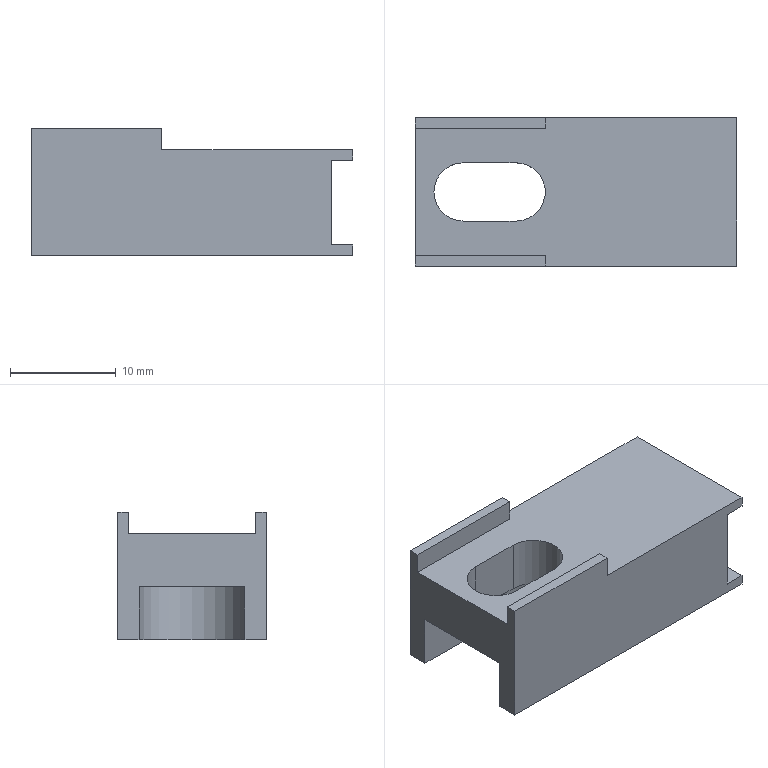Part | NX | features BREP 1 | 1 solid | 29 faces | box 30.3 x 14 x 12 mm | volume 3050 mm3 | plane 21 | cylinder 6 | cone 2 | commonest cylinder face diameters 5.5 x3 3.3 x2 10 x1
STEP:
#1=CARTESIAN_POINT('',(-758.104,11.58,6.65));
#2=VERTEX_POINT('',#1);
#3=CARTESIAN_POINT('',(-758.104,11.58,3.35));
#4=VERTEX_POINT('',#3);
#5=CARTESIAN_POINT('',(-758.104,11.58,5.));
#6=DIRECTION('',(1.,0.,0.));
#7=DIRECTION('',(0.,0.,-1.));
#8=AXIS2_PLACEMENT_3D('',#5,#6,#7);
#9=CIRCLE('',#8,1.65);
#10=EDGE_CURVE('',#2,#4,#9,.T.);
#11=ORIENTED_EDGE('',*,*,#10,.F.);
#12=CARTESIAN_POINT('',(-748.004,11.58,6.65));
#13=VERTEX_POINT('',#12);
#14=CARTESIAN_POINT('',(-748.004,11.58,6.65));
#15=DIRECTION('',(1.,0.,0.));
#16=VECTOR('',#15,1000.);
#17=LINE('',#14,#16);
#18=EDGE_CURVE('',#2,#13,#17,.T.);
#19=ORIENTED_EDGE('',*,*,#18,.T.);
#20=CARTESIAN_POINT('',(-748.004,11.58,3.35));
#21=VERTEX_POINT('',#20);
#22=CARTESIAN_POINT('',(-748.004,11.58,5.));
#23=DIRECTION('',(1.,0.,0.));
#24=DIRECTION('',(0.,0.,-1.));
#25=AXIS2_PLACEMENT_3D('',#22,#23,#24);
#26=CIRCLE('',#25,1.65);
#27=EDGE_CURVE('',#13,#21,#26,.T.);
#28=ORIENTED_EDGE('',*,*,#27,.T.);
#29=CARTESIAN_POINT('',(-748.004,11.58,3.35));
#30=DIRECTION('',(1.,0.,0.));
#31=VECTOR('',#30,1000.);
#32=LINE('',#29,#31);
#33=EDGE_CURVE('',#4,#21,#32,.T.);
#34=ORIENTED_EDGE('',*,*,#33,.F.);
#35=EDGE_LOOP('',(#11,#19,#28,#34));
#36=FACE_BOUND('',#35,.T.);
#37=CARTESIAN_POINT('',(-748.004,11.58,5.));
#38=DIRECTION('',(1.,0.,0.));
#39=DIRECTION('',(0.,0.,-1.));
#40=AXIS2_PLACEMENT_3D('',#37,#38,#39);
#41=CYLINDRICAL_SURFACE('',#40,1.65);
#42=ADVANCED_FACE('',(#36),#41,.F.);
#43=CARTESIAN_POINT('',(-759.096,11.58,5.));
#44=VERTEX_POINT('',#43);
#45=CARTESIAN_POINT('',(-758.104,11.58,3.35));
#46=DIRECTION('',(0.515,0.,-0.8572));
#47=VECTOR('',#46,1000.);
#48=LINE('',#45,#47);
#49=EDGE_CURVE('',#44,#4,#48,.T.);
#50=ORIENTED_EDGE('',*,*,#49,.F.);
#51=CARTESIAN_POINT('',(-758.104,11.58,6.65));
#52=DIRECTION('',(0.515,0.,0.8572));
#53=VECTOR('',#52,1000.);
#54=LINE('',#51,#53);
#55=EDGE_CURVE('',#44,#2,#54,.T.);
#56=ORIENTED_EDGE('',*,*,#55,.T.);
#57=ORIENTED_EDGE('',*,*,#10,.T.);
#58=EDGE_LOOP('',(#50,#56,#57));
#59=FACE_BOUND('',#58,.T.);
#60=CARTESIAN_POINT('',(-758.104,11.58,5.));
#61=DIRECTION('',(1.,0.,0.));
#62=DIRECTION('',(0.,0.,-1.));
#63=AXIS2_PLACEMENT_3D('',#60,#61,#62);
#64=CONICAL_SURFACE('',#63,1.65,1.03);
#65=ADVANCED_FACE('',(#59),#64,.F.);
#66=CARTESIAN_POINT('',(-774.554,11.58,10.));
#67=VERTEX_POINT('',#66);
#68=CARTESIAN_POINT('',(-771.804,14.33,10.));
#69=VERTEX_POINT('',#68);
#70=CARTESIAN_POINT('',(-771.804,11.58,10.));
#71=DIRECTION('',(0.,0.,-1.));
#72=DIRECTION('',(-1.,0.,0.));
#73=AXIS2_PLACEMENT_3D('',#70,#71,#72);
#74=CIRCLE('',#73,2.75);
#75=EDGE_CURVE('',#67,#69,#74,.T.);
#76=ORIENTED_EDGE('',*,*,#75,.F.);
#77=CARTESIAN_POINT('',(-774.554,11.58,5.));
#78=VERTEX_POINT('',#77);
#79=CARTESIAN_POINT('',(-774.554,11.58,12.));
#80=DIRECTION('',(0.,0.,-1.));
#81=VECTOR('',#80,1000.);
#82=LINE('',#79,#81);
#83=EDGE_CURVE('',#67,#78,#82,.T.);
#84=ORIENTED_EDGE('',*,*,#83,.T.);
#85=CARTESIAN_POINT('',(-771.804,14.33,5.));
#86=VERTEX_POINT('',#85);
#87=CARTESIAN_POINT('',(-771.804,11.58,5.));
#88=DIRECTION('',(0.,0.,1.));
#89=DIRECTION('',(-1.,0.,0.));
#90=AXIS2_PLACEMENT_3D('',#87,#88,#89);
#91=CIRCLE('',#90,2.75);
#92=EDGE_CURVE('',#86,#78,#91,.T.);
#93=ORIENTED_EDGE('',*,*,#92,.F.);
#94=CARTESIAN_POINT('',(-771.804,14.33,12.));
#95=DIRECTION('',(0.,0.,-1.));
#96=VECTOR('',#95,1000.);
#97=LINE('',#94,#96);
#98=EDGE_CURVE('',#69,#86,#97,.T.);
#99=ORIENTED_EDGE('',*,*,#98,.F.);
#100=EDGE_LOOP('',(#76,#84,#93,#99));
#101=FACE_BOUND('',#100,.T.);
#102=CARTESIAN_POINT('',(-771.804,11.58,12.));
#103=DIRECTION('',(0.,0.,-1.));
#104=DIRECTION('',(-1.,0.,0.));
#105=AXIS2_PLACEMENT_3D('',#102,#103,#104);
#106=CYLINDRICAL_SURFACE('',#105,2.75);
#107=ADVANCED_FACE('',(#101),#106,.F.);
#108=CARTESIAN_POINT('',(-776.304,16.58,0.));
#109=VERTEX_POINT('',#108);
#110=CARTESIAN_POINT('',(-776.304,16.58,5.));
#111=VERTEX_POINT('',#110);
#112=CARTESIAN_POINT('',(-776.304,16.58,0.));
#113=DIRECTION('',(0.,0.,1.));
#114=VECTOR('',#113,1000.);
#115=LINE('',#112,#114);
#116=EDGE_CURVE('',#109,#111,#115,.T.);
#117=ORIENTED_EDGE('',*,*,#116,.T.);
#118=CARTESIAN_POINT('',(-776.304,6.58,5.));
#119=VERTEX_POINT('',#118);
#120=CARTESIAN_POINT('',(-776.304,18.58,5.));
#121=DIRECTION('',(0.,1.,0.));
#122=VECTOR('',#121,1000.);
#123=LINE('',#120,#122);
#124=EDGE_CURVE('',#119,#111,#123,.T.);
#125=ORIENTED_EDGE('',*,*,#124,.F.);
#126=CARTESIAN_POINT('',(-776.304,6.58,0.));
#127=VERTEX_POINT('',#126);
#128=CARTESIAN_POINT('',(-776.304,6.58,0.));
#129=DIRECTION('',(0.,0.,1.));
#130=VECTOR('',#129,1000.);
#131=LINE('',#128,#130);
#132=EDGE_CURVE('',#127,#119,#131,.T.);
#133=ORIENTED_EDGE('',*,*,#132,.F.);
#134=CARTESIAN_POINT('',(-776.304,4.58,0.));
#135=VERTEX_POINT('',#134);
#136=CARTESIAN_POINT('',(-776.304,18.58,0.));
#137=DIRECTION('',(0.,-1.,0.));
#138=VECTOR('',#137,1000.);
#139=LINE('',#136,#138);
#140=EDGE_CURVE('',#127,#135,#139,.T.);
#141=ORIENTED_EDGE('',*,*,#140,.T.);
#142=CARTESIAN_POINT('',(-776.304,4.58,12.));
#143=VERTEX_POINT('',#142);
#144=CARTESIAN_POINT('',(-776.304,4.58,12.));
#145=DIRECTION('',(0.,0.,-1.));
#146=VECTOR('',#145,1000.);
#147=LINE('',#144,#146);
#148=EDGE_CURVE('',#143,#135,#147,.T.);
#149=ORIENTED_EDGE('',*,*,#148,.F.);
#150=CARTESIAN_POINT('',(-776.304,5.58,12.));
#151=VERTEX_POINT('',#150);
#152=CARTESIAN_POINT('',(-776.304,18.58,12.));
#153=DIRECTION('',(0.,-1.,0.));
#154=VECTOR('',#153,1000.);
#155=LINE('',#152,#154);
#156=EDGE_CURVE('',#151,#143,#155,.T.);
#157=ORIENTED_EDGE('',*,*,#156,.F.);
#158=CARTESIAN_POINT('',(-776.304,5.58,10.));
#159=VERTEX_POINT('',#158);
#160=CARTESIAN_POINT('',(-776.304,5.58,10.));
#161=DIRECTION('',(0.,0.,1.));
#162=VECTOR('',#161,1000.);
#163=LINE('',#160,#162);
#164=EDGE_CURVE('',#159,#151,#163,.T.);
#165=ORIENTED_EDGE('',*,*,#164,.F.);
#166=CARTESIAN_POINT('',(-776.304,17.58,10.));
#167=VERTEX_POINT('',#166);
#168=CARTESIAN_POINT('',(-776.304,5.58,10.));
#169=DIRECTION('',(0.,-1.,0.));
#170=VECTOR('',#169,1000.);
#171=LINE('',#168,#170);
#172=EDGE_CURVE('',#167,#159,#171,.T.);
#173=ORIENTED_EDGE('',*,*,#172,.F.);
#174=CARTESIAN_POINT('',(-776.304,17.58,12.));
#175=VERTEX_POINT('',#174);
#176=CARTESIAN_POINT('',(-776.304,17.58,10.));
#177=DIRECTION('',(0.,0.,1.));
#178=VECTOR('',#177,1000.);
#179=LINE('',#176,#178);
#180=EDGE_CURVE('',#167,#175,#179,.T.);
#181=ORIENTED_EDGE('',*,*,#180,.T.);
#182=CARTESIAN_POINT('',(-776.304,18.58,12.));
#183=VERTEX_POINT('',#182);
#184=CARTESIAN_POINT('',(-776.304,18.58,12.));
#185=DIRECTION('',(0.,-1.,0.));
#186=VECTOR('',#185,1000.);
#187=LINE('',#184,#186);
#188=EDGE_CURVE('',#183,#175,#187,.T.);
#189=ORIENTED_EDGE('',*,*,#188,.F.);
#190=CARTESIAN_POINT('',(-776.304,18.58,0.));
#191=VERTEX_POINT('',#190);
#192=CARTESIAN_POINT('',(-776.304,18.58,12.));
#193=DIRECTION('',(0.,0.,-1.));
#194=VECTOR('',#193,1000.);
#195=LINE('',#192,#194);
#196=EDGE_CURVE('',#183,#191,#195,.T.);
#197=ORIENTED_EDGE('',*,*,#196,.T.);
#198=CARTESIAN_POINT('',(-776.304,18.58,0.));
#199=DIRECTION('',(0.,-1.,0.));
#200=VECTOR('',#199,1000.);
#201=LINE('',#198,#200);
#202=EDGE_CURVE('',#191,#109,#201,.T.);
#203=ORIENTED_EDGE('',*,*,#202,.T.);
#204=EDGE_LOOP('',(#117,#125,#133,#141,#149,#157,#165,#173,#181,#189,#197,#203));
#205=FACE_BOUND('',#204,.T.);
#206=CARTESIAN_POINT('',(-776.304,18.58,12.));
#207=DIRECTION('',(1.,0.,0.));
#208=DIRECTION('',(0.,1.,0.));
#209=AXIS2_PLACEMENT_3D('',#206,#207,#208);
#210=PLANE('',#209);
#211=ADVANCED_FACE('',(#205),#210,.F.);
#212=ORIENTED_EDGE('',*,*,#140,.F.);
#213=CARTESIAN_POINT('',(-766.804,6.58,0.));
#214=VERTEX_POINT('',#213);
#215=CARTESIAN_POINT('',(-766.804,6.58,0.));
#216=DIRECTION('',(-1.,0.,0.));
#217=VECTOR('',#216,1000.);
#218=LINE('',#215,#217);
#219=EDGE_CURVE('',#214,#127,#218,.T.);
#220=ORIENTED_EDGE('',*,*,#219,.F.);
#221=CARTESIAN_POINT('',(-766.804,16.58,0.));
#222=VERTEX_POINT('',#221);
#223=CARTESIAN_POINT('',(-766.804,11.58,0.));
#224=DIRECTION('',(0.,0.,-1.));
#225=DIRECTION('',(-1.,0.,0.));
#226=AXIS2_PLACEMENT_3D('',#223,#224,#225);
#227=CIRCLE('',#226,5.);
#228=EDGE_CURVE('',#222,#214,#227,.T.);
#229=ORIENTED_EDGE('',*,*,#228,.F.);
#230=CARTESIAN_POINT('',(-771.804,16.58,0.));
#231=DIRECTION('',(1.,0.,0.));
#232=VECTOR('',#231,1000.);
#233=LINE('',#230,#232);
#234=EDGE_CURVE('',#109,#222,#233,.T.);
#235=ORIENTED_EDGE('',*,*,#234,.F.);
#236=ORIENTED_EDGE('',*,*,#202,.F.);
#237=CARTESIAN_POINT('',(-746.004,18.58,0.));
#238=VERTEX_POINT('',#237);
#239=CARTESIAN_POINT('',(-746.004,18.58,0.));
#240=DIRECTION('',(-1.,0.,0.));
#241=VECTOR('',#240,1000.);
#242=LINE('',#239,#241);
#243=EDGE_CURVE('',#238,#191,#242,.T.);
#244=ORIENTED_EDGE('',*,*,#243,.F.);
#245=CARTESIAN_POINT('',(-746.004,4.58,0.));
#246=VERTEX_POINT('',#245);
#247=CARTESIAN_POINT('',(-746.004,18.58,0.));
#248=DIRECTION('',(0.,1.,0.));
#249=VECTOR('',#248,1000.);
#250=LINE('',#247,#249);
#251=EDGE_CURVE('',#246,#238,#250,.T.);
#252=ORIENTED_EDGE('',*,*,#251,.F.);
#253=CARTESIAN_POINT('',(-746.004,4.58,0.));
#254=DIRECTION('',(1.,0.,0.));
#255=VECTOR('',#254,1000.);
#256=LINE('',#253,#255);
#257=EDGE_CURVE('',#135,#246,#256,.T.);
#258=ORIENTED_EDGE('',*,*,#257,.F.);
#259=EDGE_LOOP('',(#212,#220,#229,#235,#236,#244,#252,#258));
#260=FACE_BOUND('',#259,.T.);
#261=CARTESIAN_POINT('',(-746.004,4.58,0.));
#262=DIRECTION('',(0.,0.,-1.));
#263=DIRECTION('',(0.,-1.,0.));
#264=AXIS2_PLACEMENT_3D('',#261,#262,#263);
#265=PLANE('',#264);
#266=ADVANCED_FACE('',(#260),#265,.T.);
#267=CARTESIAN_POINT('',(-766.804,8.83,5.));
#268=VERTEX_POINT('',#267);
#269=CARTESIAN_POINT('',(-766.804,14.33,5.));
#270=VERTEX_POINT('',#269);
#271=CARTESIAN_POINT('',(-766.804,11.58,5.));
#272=DIRECTION('',(0.,0.,1.));
#273=DIRECTION('',(-1.,0.,0.));
#274=AXIS2_PLACEMENT_3D('',#271,#272,#273);
#275=CIRCLE('',#274,2.75);
#276=EDGE_CURVE('',#268,#270,#275,.T.);
#277=ORIENTED_EDGE('',*,*,#276,.F.);
#278=CARTESIAN_POINT('',(-766.804,8.83,10.));
#279=VERTEX_POINT('',#278);
#280=CARTESIAN_POINT('',(-766.804,8.83,12.));
#281=DIRECTION('',(0.,0.,-1.));
#282=VECTOR('',#281,1000.);
#283=LINE('',#280,#282);
#284=EDGE_CURVE('',#279,#268,#283,.T.);
#285=ORIENTED_EDGE('',*,*,#284,.F.);
#286=CARTESIAN_POINT('',(-766.804,14.33,10.));
#287=VERTEX_POINT('',#286);
#288=CARTESIAN_POINT('',(-766.804,11.58,10.));
#289=DIRECTION('',(0.,0.,-1.));
#290=DIRECTION('',(-1.,0.,0.));
#291=AXIS2_PLACEMENT_3D('',#288,#289,#290);
#292=CIRCLE('',#291,2.75);
#293=EDGE_CURVE('',#287,#279,#292,.T.);
#294=ORIENTED_EDGE('',*,*,#293,.F.);
#295=CARTESIAN_POINT('',(-766.804,14.33,12.));
#296=DIRECTION('',(0.,0.,-1.));
#297=VECTOR('',#296,1000.);
#298=LINE('',#295,#297);
#299=EDGE_CURVE('',#287,#270,#298,.T.);
#300=ORIENTED_EDGE('',*,*,#299,.T.);
#301=EDGE_LOOP('',(#277,#285,#294,#300));
#302=FACE_BOUND('',#301,.T.);
#303=CARTESIAN_POINT('',(-766.804,11.58,12.));
#304=DIRECTION('',(0.,0.,-1.));
#305=DIRECTION('',(-1.,0.,0.));
#306=AXIS2_PLACEMENT_3D('',#303,#304,#305);
#307=CYLINDRICAL_SURFACE('',#306,2.75);
#308=ADVANCED_FACE('',(#302),#307,.F.);
#309=CARTESIAN_POINT('',(-766.804,14.33,5.));
#310=DIRECTION('',(-1.,0.,0.));
#311=VECTOR('',#310,1000.);
#312=LINE('',#309,#311);
#313=EDGE_CURVE('',#270,#86,#312,.T.);
#314=ORIENTED_EDGE('',*,*,#313,.F.);
#315=ORIENTED_EDGE('',*,*,#299,.F.);
#316=CARTESIAN_POINT('',(-776.304,14.33,10.));
#317=DIRECTION('',(1.,0.,0.));
#318=VECTOR('',#317,1000.);
#319=LINE('',#316,#318);
#320=EDGE_CURVE('',#69,#287,#319,.T.);
#321=ORIENTED_EDGE('',*,*,#320,.F.);
#322=ORIENTED_EDGE('',*,*,#98,.T.);
#323=EDGE_LOOP('',(#314,#315,#321,#322));
#324=FACE_BOUND('',#323,.T.);
#325=CARTESIAN_POINT('',(-766.804,14.33,12.));
#326=DIRECTION('',(0.,1.,0.));
#327=DIRECTION('',(1.,0.,0.));
#328=AXIS2_PLACEMENT_3D('',#325,#326,#327);
#329=PLANE('',#328);
#330=ADVANCED_FACE('',(#324),#329,.F.);
#331=ORIENTED_EDGE('',*,*,#83,.F.);
#332=CARTESIAN_POINT('',(-771.804,8.83,10.));
#333=VERTEX_POINT('',#332);
#334=CARTESIAN_POINT('',(-771.804,11.58,10.));
#335=DIRECTION('',(0.,0.,-1.));
#336=DIRECTION('',(-1.,0.,0.));
#337=AXIS2_PLACEMENT_3D('',#334,#335,#336);
#338=CIRCLE('',#337,2.75);
#339=EDGE_CURVE('',#333,#67,#338,.T.);
#340=ORIENTED_EDGE('',*,*,#339,.F.);
#341=CARTESIAN_POINT('',(-771.804,8.83,5.));
#342=VERTEX_POINT('',#341);
#343=CARTESIAN_POINT('',(-771.804,8.83,12.));
#344=DIRECTION('',(0.,0.,-1.));
#345=VECTOR('',#344,1000.);
#346=LINE('',#343,#345);
#347=EDGE_CURVE('',#333,#342,#346,.T.);
#348=ORIENTED_EDGE('',*,*,#347,.T.);
#349=CARTESIAN_POINT('',(-771.804,11.58,5.));
#350=DIRECTION('',(0.,0.,1.));
#351=DIRECTION('',(-1.,0.,0.));
#352=AXIS2_PLACEMENT_3D('',#349,#350,#351);
#353=CIRCLE('',#352,2.75);
#354=EDGE_CURVE('',#78,#342,#353,.T.);
#355=ORIENTED_EDGE('',*,*,#354,.F.);
#356=EDGE_LOOP('',(#331,#340,#348,#355));
#357=FACE_BOUND('',#356,.T.);
#358=CARTESIAN_POINT('',(-771.804,11.58,12.));
#359=DIRECTION('',(0.,0.,-1.));
#360=DIRECTION('',(-1.,0.,0.));
#361=AXIS2_PLACEMENT_3D('',#358,#359,#360);
#362=CYLINDRICAL_SURFACE('',#361,2.75);
#363=ADVANCED_FACE('',(#357),#362,.F.);
#364=CARTESIAN_POINT('',(-766.804,8.83,5.));
#365=DIRECTION('',(1.,0.,0.));
#366=VECTOR('',#365,1000.);
#367=LINE('',#364,#366);
#368=EDGE_CURVE('',#342,#268,#367,.T.);
#369=ORIENTED_EDGE('',*,*,#368,.F.);
#370=ORIENTED_EDGE('',*,*,#347,.F.);
#371=CARTESIAN_POINT('',(-776.304,8.83,10.));
#372=DIRECTION('',(-1.,0.,0.));
#373=VECTOR('',#372,1000.);
#374=LINE('',#371,#373);
#375=EDGE_CURVE('',#279,#333,#374,.T.);
#376=ORIENTED_EDGE('',*,*,#375,.F.);
#377=ORIENTED_EDGE('',*,*,#284,.T.);
#378=EDGE_LOOP('',(#369,#370,#376,#377));
#379=FACE_BOUND('',#378,.T.);
#380=CARTESIAN_POINT('',(-766.804,8.83,12.));
#381=DIRECTION('',(0.,-1.,0.));
#382=DIRECTION('',(0.,0.,-1.));
#383=AXIS2_PLACEMENT_3D('',#380,#381,#382);
#384=PLANE('',#383);
#385=ADVANCED_FACE('',(#379),#384,.F.);
#386=CARTESIAN_POINT('',(-746.004,18.58,1.));
#387=VERTEX_POINT('',#386);
#388=CARTESIAN_POINT('',(-746.004,18.58,12.));
#389=DIRECTION('',(0.,0.,-1.));
#390=VECTOR('',#389,1000.);
#391=LINE('',#388,#390);
#392=EDGE_CURVE('',#387,#238,#391,.T.);
#393=ORIENTED_EDGE('',*,*,#392,.F.);
#394=CARTESIAN_POINT('',(-746.004,4.58,1.));
#395=VERTEX_POINT('',#394);
#396=CARTESIAN_POINT('',(-746.004,18.58,1.));
#397=DIRECTION('',(0.,1.,0.));
#398=VECTOR('',#397,1000.);
#399=LINE('',#396,#398);
#400=EDGE_CURVE('',#395,#387,#399,.T.);
#401=ORIENTED_EDGE('',*,*,#400,.F.);
#402=CARTESIAN_POINT('',(-746.004,4.58,12.));
#403=DIRECTION('',(0.,0.,-1.));
#404=VECTOR('',#403,1000.);
#405=LINE('',#402,#404);
#406=EDGE_CURVE('',#395,#246,#405,.T.);
#407=ORIENTED_EDGE('',*,*,#406,.T.);
#408=ORIENTED_EDGE('',*,*,#251,.T.);
#409=EDGE_LOOP('',(#393,#401,#407,#408));
#410=FACE_BOUND('',#409,.T.);
#411=CARTESIAN_POINT('',(-746.004,18.58,12.));
#412=DIRECTION('',(-1.,0.,0.));
#413=DIRECTION('',(0.,0.,1.));
#414=AXIS2_PLACEMENT_3D('',#411,#412,#413);
#415=PLANE('',#414);
#416=ADVANCED_FACE('',(#410),#415,.F.);
#417=CARTESIAN_POINT('',(-764.004,17.58,12.));
#418=VERTEX_POINT('',#417);
#419=CARTESIAN_POINT('',(-776.304,17.58,12.));
#420=DIRECTION('',(-1.,0.,0.));
#421=VECTOR('',#420,1000.);
#422=LINE('',#419,#421);
#423=EDGE_CURVE('',#418,#175,#422,.T.);
#424=ORIENTED_EDGE('',*,*,#423,.F.);
#425=CARTESIAN_POINT('',(-764.004,18.58,12.));
#426=VERTEX_POINT('',#425);
#427=CARTESIAN_POINT('',(-764.004,18.58,12.));
#428=DIRECTION('',(0.,-1.,0.));
#429=VECTOR('',#428,1000.);
#430=LINE('',#427,#429);
#431=EDGE_CURVE('',#426,#418,#430,.T.);
#432=ORIENTED_EDGE('',*,*,#431,.F.);
#433=CARTESIAN_POINT('',(-746.004,18.58,12.));
#434=DIRECTION('',(-1.,0.,0.));
#435=VECTOR('',#434,1000.);
#436=LINE('',#433,#435);
#437=EDGE_CURVE('',#426,#183,#436,.T.);
#438=ORIENTED_EDGE('',*,*,#437,.T.);
#439=ORIENTED_EDGE('',*,*,#188,.T.);
#440=EDGE_LOOP('',(#424,#432,#438,#439));
#441=FACE_BOUND('',#440,.T.);
#442=CARTESIAN_POINT('',(-746.004,4.58,12.));
#443=DIRECTION('',(0.,0.,-1.));
#444=DIRECTION('',(0.,-1.,0.));
#445=AXIS2_PLACEMENT_3D('',#442,#443,#444);
#446=PLANE('',#445);
#447=ADVANCED_FACE('',(#441),#446,.F.);
#448=CARTESIAN_POINT('',(-746.004,18.58,10.));
#449=VERTEX_POINT('',#448);
#450=CARTESIAN_POINT('',(-746.004,18.58,9.));
#451=VERTEX_POINT('',#450);
#452=CARTESIAN_POINT('',(-746.004,18.58,12.));
#453=DIRECTION('',(0.,0.,-1.));
#454=VECTOR('',#453,1000.);
#455=LINE('',#452,#454);
#456=EDGE_CURVE('',#449,#451,#455,.T.);
#457=ORIENTED_EDGE('',*,*,#456,.F.);
#458=CARTESIAN_POINT('',(-746.004,4.58,10.));
#459=VERTEX_POINT('',#458);
#460=CARTESIAN_POINT('',(-746.004,5.58,10.));
#461=DIRECTION('',(0.,1.,0.));
#462=VECTOR('',#461,1000.);
#463=LINE('',#460,#462);
#464=EDGE_CURVE('',#459,#449,#463,.T.);
#465=ORIENTED_EDGE('',*,*,#464,.F.);
#466=CARTESIAN_POINT('',(-746.004,4.58,9.));
#467=VERTEX_POINT('',#466);
#468=CARTESIAN_POINT('',(-746.004,4.58,12.));
#469=DIRECTION('',(0.,0.,-1.));
#470=VECTOR('',#469,1000.);
#471=LINE('',#468,#470);
#472=EDGE_CURVE('',#459,#467,#471,.T.);
#473=ORIENTED_EDGE('',*,*,#472,.T.);
#474=CARTESIAN_POINT('',(-746.004,18.58,9.));
#475=DIRECTION('',(0.,-1.,0.));
#476=VECTOR('',#475,1000.);
#477=LINE('',#474,#476);
#478=EDGE_CURVE('',#451,#467,#477,.T.);
#479=ORIENTED_EDGE('',*,*,#478,.F.);
#480=EDGE_LOOP('',(#457,#465,#473,#479));
#481=FACE_BOUND('',#480,.T.);
#482=CARTESIAN_POINT('',(-746.004,18.58,12.));
#483=DIRECTION('',(-1.,0.,0.));
#484=DIRECTION('',(0.,0.,1.));
#485=AXIS2_PLACEMENT_3D('',#482,#483,#484);
#486=PLANE('',#485);
#487=ADVANCED_FACE('',(#481),#486,.F.);
#488=CARTESIAN_POINT('',(-764.004,18.58,10.));
#489=VERTEX_POINT('',#488);
#490=CARTESIAN_POINT('',(-764.004,18.58,12.));
#491=DIRECTION('',(0.,0.,-1.));
#492=VECTOR('',#491,1000.);
#493=LINE('',#490,#492);
#494=EDGE_CURVE('',#426,#489,#493,.T.);
#495=ORIENTED_EDGE('',*,*,#494,.T.);
#496=CARTESIAN_POINT('',(-746.004,18.58,10.));
#497=DIRECTION('',(1.,0.,0.));
#498=VECTOR('',#497,1000.);
#499=LINE('',#496,#498);
#500=EDGE_CURVE('',#489,#449,#499,.T.);
#501=ORIENTED_EDGE('',*,*,#500,.T.);
#502=ORIENTED_EDGE('',*,*,#456,.T.);
#503=CARTESIAN_POINT('',(-748.004,18.58,9.));
#504=VERTEX_POINT('',#503);
#505=CARTESIAN_POINT('',(-748.004,18.58,9.));
#506=DIRECTION('',(1.,0.,0.));
#507=VECTOR('',#506,1000.);
#508=LINE('',#505,#507);
#509=EDGE_CURVE('',#504,#451,#508,.T.);
#510=ORIENTED_EDGE('',*,*,#509,.F.);
#511=CARTESIAN_POINT('',(-748.004,18.58,1.));
#512=VERTEX_POINT('',#511);
#513=CARTESIAN_POINT('',(-748.004,18.58,1.));
#514=DIRECTION('',(0.,0.,1.));
#515=VECTOR('',#514,1000.);
#516=LINE('',#513,#515);
#517=EDGE_CURVE('',#512,#504,#516,.T.);
#518=ORIENTED_EDGE('',*,*,#517,.F.);
#519=CARTESIAN_POINT('',(-748.004,18.58,1.));
#520=DIRECTION('',(1.,0.,0.));
#521=VECTOR('',#520,1000.);
#522=LINE('',#519,#521);
#523=EDGE_CURVE('',#512,#387,#522,.T.);
#524=ORIENTED_EDGE('',*,*,#523,.T.);
#525=ORIENTED_EDGE('',*,*,#392,.T.);
#526=ORIENTED_EDGE('',*,*,#243,.T.);
#527=ORIENTED_EDGE('',*,*,#196,.F.);
#528=ORIENTED_EDGE('',*,*,#437,.F.);
#529=EDGE_LOOP('',(#495,#501,#502,#510,#518,#524,#525,#526,#527,#528));
#530=FACE_BOUND('',#529,.T.);
#531=CARTESIAN_POINT('',(-746.004,18.58,12.));
#532=DIRECTION('',(0.,-1.,0.));
#533=DIRECTION('',(0.,0.,-1.));
#534=AXIS2_PLACEMENT_3D('',#531,#532,#533);
#535=PLANE('',#534);
#536=ADVANCED_FACE('',(#530),#535,.F.);
#537=ORIENTED_EDGE('',*,*,#472,.F.);
#538=CARTESIAN_POINT('',(-764.004,4.58,10.));
#539=VERTEX_POINT('',#538);
#540=CARTESIAN_POINT('',(-746.004,4.58,10.));
#541=DIRECTION('',(1.,0.,0.));
#542=VECTOR('',#541,1000.);
#543=LINE('',#540,#542);
#544=EDGE_CURVE('',#539,#459,#543,.T.);
#545=ORIENTED_EDGE('',*,*,#544,.F.);
#546=CARTESIAN_POINT('',(-764.004,4.58,12.));
#547=VERTEX_POINT('',#546);
#548=CARTESIAN_POINT('',(-764.004,4.58,12.));
#549=DIRECTION('',(0.,0.,-1.));
#550=VECTOR('',#549,1000.);
#551=LINE('',#548,#550);
#552=EDGE_CURVE('',#547,#539,#551,.T.);
#553=ORIENTED_EDGE('',*,*,#552,.F.);
#554=CARTESIAN_POINT('',(-746.004,4.58,12.));
#555=DIRECTION('',(1.,0.,0.));
#556=VECTOR('',#555,1000.);
#557=LINE('',#554,#556);
#558=EDGE_CURVE('',#143,#547,#557,.T.);
#559=ORIENTED_EDGE('',*,*,#558,.F.);
#560=ORIENTED_EDGE('',*,*,#148,.T.);
#561=ORIENTED_EDGE('',*,*,#257,.T.);
#562=ORIENTED_EDGE('',*,*,#406,.F.);
#563=CARTESIAN_POINT('',(-748.004,4.58,1.));
#564=VERTEX_POINT('',#563);
#565=CARTESIAN_POINT('',(-748.004,4.58,1.));
#566=DIRECTION('',(1.,0.,0.));
#567=VECTOR('',#566,1000.);
#568=LINE('',#565,#567);
#569=EDGE_CURVE('',#564,#395,#568,.T.);
#570=ORIENTED_EDGE('',*,*,#569,.F.);
#571=CARTESIAN_POINT('',(-748.004,4.58,9.));
#572=VERTEX_POINT('',#571);
#573=CARTESIAN_POINT('',(-748.004,4.58,1.));
#574=DIRECTION('',(0.,0.,-1.));
#575=VECTOR('',#574,1000.);
#576=LINE('',#573,#575);
#577=EDGE_CURVE('',#572,#564,#576,.T.);
#578=ORIENTED_EDGE('',*,*,#577,.F.);
#579=CARTESIAN_POINT('',(-748.004,4.58,9.));
#580=DIRECTION('',(1.,0.,0.));
#581=VECTOR('',#580,1000.);
#582=LINE('',#579,#581);
#583=EDGE_CURVE('',#572,#467,#582,.T.);
#584=ORIENTED_EDGE('',*,*,#583,.T.);
#585=EDGE_LOOP('',(#537,#545,#553,#559,#560,#561,#562,#570,#578,#584));
#586=FACE_BOUND('',#585,.T.);
#587=CARTESIAN_POINT('',(-746.004,4.58,12.));
#588=DIRECTION('',(0.,1.,0.));
#589=DIRECTION('',(1.,0.,0.));
#590=AXIS2_PLACEMENT_3D('',#587,#588,#589);
#591=PLANE('',#590);
#592=ADVANCED_FACE('',(#586),#591,.F.);
#593=ORIENTED_EDGE('',*,*,#558,.T.);
#594=CARTESIAN_POINT('',(-764.004,5.58,12.));
#595=VERTEX_POINT('',#594);
#596=CARTESIAN_POINT('',(-764.004,18.58,12.));
#597=DIRECTION('',(0.,-1.,0.));
#598=VECTOR('',#597,1000.);
#599=LINE('',#596,#598);
#600=EDGE_CURVE('',#595,#547,#599,.T.);
#601=ORIENTED_EDGE('',*,*,#600,.F.);
#602=CARTESIAN_POINT('',(-776.304,5.58,12.));
#603=DIRECTION('',(1.,0.,0.));
#604=VECTOR('',#603,1000.);
#605=LINE('',#602,#604);
#606=EDGE_CURVE('',#151,#595,#605,.T.);
#607=ORIENTED_EDGE('',*,*,#606,.F.);
#608=ORIENTED_EDGE('',*,*,#156,.T.);
#609=EDGE_LOOP('',(#593,#601,#607,#608));
#610=FACE_BOUND('',#609,.T.);
#611=CARTESIAN_POINT('',(-746.004,4.58,12.));
#612=DIRECTION('',(0.,0.,-1.));
#613=DIRECTION('',(0.,-1.,0.));
#614=AXIS2_PLACEMENT_3D('',#611,#612,#613);
#615=PLANE('',#614);
#616=ADVANCED_FACE('',(#610),#615,.F.);
#617=CARTESIAN_POINT('',(-764.004,17.58,10.));
#618=VERTEX_POINT('',#617);
#619=CARTESIAN_POINT('',(-776.304,17.58,10.));
#620=DIRECTION('',(-1.,0.,0.));
#621=VECTOR('',#620,1000.);
#622=LINE('',#619,#621);
#623=EDGE_CURVE('',#618,#167,#622,.T.);
#624=ORIENTED_EDGE('',*,*,#623,.F.);
#625=CARTESIAN_POINT('',(-764.004,17.58,10.));
#626=DIRECTION('',(0.,0.,1.));
#627=VECTOR('',#626,1000.);
#628=LINE('',#625,#627);
#629=EDGE_CURVE('',#618,#418,#628,.T.);
#630=ORIENTED_EDGE('',*,*,#629,.T.);
#631=ORIENTED_EDGE('',*,*,#423,.T.);
#632=ORIENTED_EDGE('',*,*,#180,.F.);
#633=EDGE_LOOP('',(#624,#630,#631,#632));
#634=FACE_BOUND('',#633,.T.);
#635=CARTESIAN_POINT('',(-776.304,17.58,10.));
#636=DIRECTION('',(0.,1.,0.));
#637=DIRECTION('',(1.,0.,0.));
#638=AXIS2_PLACEMENT_3D('',#635,#636,#637);
#639=PLANE('',#638);
#640=ADVANCED_FACE('',(#634),#639,.F.);
#641=ORIENTED_EDGE('',*,*,#606,.T.);
#642=CARTESIAN_POINT('',(-764.004,5.58,10.));
#643=VERTEX_POINT('',#642);
#644=CARTESIAN_POINT('',(-764.004,5.58,10.));
#645=DIRECTION('',(0.,0.,-1.));
#646=VECTOR('',#645,1000.);
#647=LINE('',#644,#646);
#648=EDGE_CURVE('',#595,#643,#647,.T.);
#649=ORIENTED_EDGE('',*,*,#648,.T.);
#650=CARTESIAN_POINT('',(-776.304,5.58,10.));
#651=DIRECTION('',(1.,0.,0.));
#652=VECTOR('',#651,1000.);
#653=LINE('',#650,#652);
#654=EDGE_CURVE('',#159,#643,#653,.T.);
#655=ORIENTED_EDGE('',*,*,#654,.F.);
#656=ORIENTED_EDGE('',*,*,#164,.T.);
#657=EDGE_LOOP('',(#641,#649,#655,#656));
#658=FACE_BOUND('',#657,.T.);
#659=CARTESIAN_POINT('',(-776.304,5.58,10.));
#660=DIRECTION('',(0.,-1.,0.));
#661=DIRECTION('',(0.,0.,-1.));
#662=AXIS2_PLACEMENT_3D('',#659,#660,#661);
#663=PLANE('',#662);
#664=ADVANCED_FACE('',(#658),#663,.F.);
#665=ORIENTED_EDGE('',*,*,#654,.T.);
#666=CARTESIAN_POINT('',(-764.004,18.58,10.));
#667=DIRECTION('',(0.,-1.,0.));
#668=VECTOR('',#667,1000.);
#669=LINE('',#666,#668);
#670=EDGE_CURVE('',#643,#539,#669,.T.);
#671=ORIENTED_EDGE('',*,*,#670,.T.);
#672=ORIENTED_EDGE('',*,*,#544,.T.);
#673=ORIENTED_EDGE('',*,*,#464,.T.);
#674=ORIENTED_EDGE('',*,*,#500,.F.);
#675=CARTESIAN_POINT('',(-764.004,18.58,10.));
#676=DIRECTION('',(0.,-1.,0.));
#677=VECTOR('',#676,1000.);
#678=LINE('',#675,#677);
#679=EDGE_CURVE('',#489,#618,#678,.T.);
#680=ORIENTED_EDGE('',*,*,#679,.T.);
#681=ORIENTED_EDGE('',*,*,#623,.T.);
#682=ORIENTED_EDGE('',*,*,#172,.T.);
#683=EDGE_LOOP('',(#665,#671,#672,#673,#674,#680,#681,#682));
#684=FACE_BOUND('',#683,.T.);
#685=ORIENTED_EDGE('',*,*,#320,.T.);
#686=ORIENTED_EDGE('',*,*,#293,.T.);
#687=ORIENTED_EDGE('',*,*,#375,.T.);
#688=ORIENTED_EDGE('',*,*,#339,.T.);
#689=ORIENTED_EDGE('',*,*,#75,.T.);
#690=EDGE_LOOP('',(#685,#686,#687,#688,#689));
#691=FACE_BOUND('',#690,.T.);
#692=CARTESIAN_POINT('',(-776.304,17.58,10.));
#693=DIRECTION('',(0.,0.,-1.));
#694=DIRECTION('',(0.,-1.,0.));
#695=AXIS2_PLACEMENT_3D('',#692,#693,#694);
#696=PLANE('',#695);
#697=ADVANCED_FACE('',(#684,#691),#696,.F.);
#698=ORIENTED_EDGE('',*,*,#400,.T.);
#699=ORIENTED_EDGE('',*,*,#523,.F.);
#700=CARTESIAN_POINT('',(-748.004,18.58,1.));
#701=DIRECTION('',(0.,1.,0.));
#702=VECTOR('',#701,1000.);
#703=LINE('',#700,#702);
#704=EDGE_CURVE('',#564,#512,#703,.T.);
#705=ORIENTED_EDGE('',*,*,#704,.F.);
#706=ORIENTED_EDGE('',*,*,#569,.T.);
#707=EDGE_LOOP('',(#698,#699,#705,#706));
#708=FACE_BOUND('',#707,.T.);
#709=CARTESIAN_POINT('',(-748.004,18.58,1.));
#710=DIRECTION('',(0.,0.,-1.));
#711=DIRECTION('',(-1.,0.,0.));
#712=AXIS2_PLACEMENT_3D('',#709,#710,#711);
#713=PLANE('',#712);
#714=ADVANCED_FACE('',(#708),#713,.F.);
#715=ORIENTED_EDGE('',*,*,#478,.T.);
#716=ORIENTED_EDGE('',*,*,#583,.F.);
#717=CARTESIAN_POINT('',(-748.004,18.58,9.));
#718=DIRECTION('',(0.,-1.,0.));
#719=VECTOR('',#718,1000.);
#720=LINE('',#717,#719);
#721=EDGE_CURVE('',#504,#572,#720,.T.);
#722=ORIENTED_EDGE('',*,*,#721,.F.);
#723=ORIENTED_EDGE('',*,*,#509,.T.);
#724=EDGE_LOOP('',(#715,#716,#722,#723));
#725=FACE_BOUND('',#724,.T.);
#726=CARTESIAN_POINT('',(-748.004,18.58,9.));
#727=DIRECTION('',(0.,0.,1.));
#728=DIRECTION('',(0.,-1.,0.));
#729=AXIS2_PLACEMENT_3D('',#726,#727,#728);
#730=PLANE('',#729);
#731=ADVANCED_FACE('',(#725),#730,.F.);
#732=ORIENTED_EDGE('',*,*,#704,.T.);
#733=ORIENTED_EDGE('',*,*,#517,.T.);
#734=ORIENTED_EDGE('',*,*,#721,.T.);
#735=ORIENTED_EDGE('',*,*,#577,.T.);
#736=EDGE_LOOP('',(#732,#733,#734,#735));
#737=FACE_BOUND('',#736,.T.);
#738=CARTESIAN_POINT('',(-748.004,11.58,5.));
#739=DIRECTION('',(1.,0.,0.));
#740=DIRECTION('',(0.,0.,-1.));
#741=AXIS2_PLACEMENT_3D('',#738,#739,#740);
#742=CIRCLE('',#741,1.65);
#743=EDGE_CURVE('',#21,#13,#742,.T.);
#744=ORIENTED_EDGE('',*,*,#743,.F.);
#745=ORIENTED_EDGE('',*,*,#27,.F.);
#746=EDGE_LOOP('',(#744,#745));
#747=FACE_BOUND('',#746,.T.);
#748=CARTESIAN_POINT('',(-748.004,4.58,1.));
#749=DIRECTION('',(-1.,0.,0.));
#750=DIRECTION('',(0.,0.,1.));
#751=AXIS2_PLACEMENT_3D('',#748,#749,#750);
#752=PLANE('',#751);
#753=ADVANCED_FACE('',(#737,#747),#752,.F.);
#754=ORIENTED_EDGE('',*,*,#600,.T.);
#755=ORIENTED_EDGE('',*,*,#552,.T.);
#756=ORIENTED_EDGE('',*,*,#670,.F.);
#757=ORIENTED_EDGE('',*,*,#648,.F.);
#758=EDGE_LOOP('',(#754,#755,#756,#757));
#759=FACE_BOUND('',#758,.T.);
#760=CARTESIAN_POINT('',(-764.004,18.58,12.));
#761=DIRECTION('',(-1.,0.,0.));
#762=DIRECTION('',(0.,1.,0.));
#763=AXIS2_PLACEMENT_3D('',#760,#761,#762);
#764=PLANE('',#763);
#765=ADVANCED_FACE('',(#759),#764,.F.);
#766=ORIENTED_EDGE('',*,*,#679,.F.);
#767=ORIENTED_EDGE('',*,*,#494,.F.);
#768=ORIENTED_EDGE('',*,*,#431,.T.);
#769=ORIENTED_EDGE('',*,*,#629,.F.);
#770=EDGE_LOOP('',(#766,#767,#768,#769));
#771=FACE_BOUND('',#770,.T.);
#772=CARTESIAN_POINT('',(-764.004,18.58,12.));
#773=DIRECTION('',(-1.,0.,0.));
#774=DIRECTION('',(0.,1.,0.));
#775=AXIS2_PLACEMENT_3D('',#772,#773,#774);
#776=PLANE('',#775);
#777=ADVANCED_FACE('',(#771),#776,.F.);
#778=ORIENTED_EDGE('',*,*,#55,.F.);
#779=ORIENTED_EDGE('',*,*,#49,.T.);
#780=CARTESIAN_POINT('',(-758.104,11.58,5.));
#781=DIRECTION('',(1.,0.,0.));
#782=DIRECTION('',(0.,0.,-1.));
#783=AXIS2_PLACEMENT_3D('',#780,#781,#782);
#784=CIRCLE('',#783,1.65);
#785=EDGE_CURVE('',#4,#2,#784,.T.);
#786=ORIENTED_EDGE('',*,*,#785,.T.);
#787=EDGE_LOOP('',(#778,#779,#786));
#788=FACE_BOUND('',#787,.T.);
#789=CARTESIAN_POINT('',(-758.104,11.58,5.));
#790=DIRECTION('',(1.,0.,0.));
#791=DIRECTION('',(0.,0.,-1.));
#792=AXIS2_PLACEMENT_3D('',#789,#790,#791);
#793=CONICAL_SURFACE('',#792,1.65,1.03);
#794=ADVANCED_FACE('',(#788),#793,.F.);
#795=ORIENTED_EDGE('',*,*,#18,.F.);
#796=ORIENTED_EDGE('',*,*,#785,.F.);
#797=ORIENTED_EDGE('',*,*,#33,.T.);
#798=ORIENTED_EDGE('',*,*,#743,.T.);
#799=EDGE_LOOP('',(#795,#796,#797,#798));
#800=FACE_BOUND('',#799,.T.);
#801=CARTESIAN_POINT('',(-748.004,11.58,5.));
#802=DIRECTION('',(1.,0.,0.));
#803=DIRECTION('',(0.,0.,-1.));
#804=AXIS2_PLACEMENT_3D('',#801,#802,#803);
#805=CYLINDRICAL_SURFACE('',#804,1.65);
#806=ADVANCED_FACE('',(#800),#805,.F.);
#807=CARTESIAN_POINT('',(-766.804,6.58,5.));
#808=VERTEX_POINT('',#807);
#809=CARTESIAN_POINT('',(-766.804,6.58,5.));
#810=DIRECTION('',(-1.,0.,0.));
#811=VECTOR('',#810,1000.);
#812=LINE('',#809,#811);
#813=EDGE_CURVE('',#808,#119,#812,.T.);
#814=ORIENTED_EDGE('',*,*,#813,.T.);
#815=ORIENTED_EDGE('',*,*,#124,.T.);
#816=CARTESIAN_POINT('',(-766.804,16.58,5.));
#817=VERTEX_POINT('',#816);
#818=CARTESIAN_POINT('',(-771.804,16.58,5.));
#819=DIRECTION('',(1.,0.,0.));
#820=VECTOR('',#819,1000.);
#821=LINE('',#818,#820);
#822=EDGE_CURVE('',#111,#817,#821,.T.);
#823=ORIENTED_EDGE('',*,*,#822,.T.);
#824=CARTESIAN_POINT('',(-766.804,11.58,5.));
#825=DIRECTION('',(0.,0.,-1.));
#826=DIRECTION('',(-1.,0.,0.));
#827=AXIS2_PLACEMENT_3D('',#824,#825,#826);
#828=CIRCLE('',#827,5.);
#829=EDGE_CURVE('',#817,#808,#828,.T.);
#830=ORIENTED_EDGE('',*,*,#829,.T.);
#831=EDGE_LOOP('',(#814,#815,#823,#830));
#832=FACE_BOUND('',#831,.T.);
#833=ORIENTED_EDGE('',*,*,#92,.T.);
#834=ORIENTED_EDGE('',*,*,#354,.T.);
#835=ORIENTED_EDGE('',*,*,#368,.T.);
#836=ORIENTED_EDGE('',*,*,#276,.T.);
#837=ORIENTED_EDGE('',*,*,#313,.T.);
#838=EDGE_LOOP('',(#833,#834,#835,#836,#837));
#839=FACE_BOUND('',#838,.T.);
#840=CARTESIAN_POINT('',(-771.804,11.58,5.));
#841=DIRECTION('',(0.,0.,-1.));
#842=DIRECTION('',(0.,-1.,0.));
#843=AXIS2_PLACEMENT_3D('',#840,#841,#842);
#844=PLANE('',#843);
#845=ADVANCED_FACE('',(#832,#839),#844,.T.);
#846=ORIENTED_EDGE('',*,*,#219,.T.);
#847=ORIENTED_EDGE('',*,*,#132,.T.);
#848=ORIENTED_EDGE('',*,*,#813,.F.);
#849=CARTESIAN_POINT('',(-766.804,6.58,5.));
#850=DIRECTION('',(0.,0.,-1.));
#851=VECTOR('',#850,1000.);
#852=LINE('',#849,#851);
#853=EDGE_CURVE('',#808,#214,#852,.T.);
#854=ORIENTED_EDGE('',*,*,#853,.T.);
#855=EDGE_LOOP('',(#846,#847,#848,#854));
#856=FACE_BOUND('',#855,.T.);
#857=CARTESIAN_POINT('',(-766.804,6.58,5.));
#858=DIRECTION('',(0.,-1.,0.));
#859=DIRECTION('',(-1.,0.,0.));
#860=AXIS2_PLACEMENT_3D('',#857,#858,#859);
#861=PLANE('',#860);
#862=ADVANCED_FACE('',(#856),#861,.F.);
#863=ORIENTED_EDGE('',*,*,#228,.T.);
#864=ORIENTED_EDGE('',*,*,#853,.F.);
#865=ORIENTED_EDGE('',*,*,#829,.F.);
#866=CARTESIAN_POINT('',(-766.804,16.58,5.));
#867=DIRECTION('',(0.,0.,-1.));
#868=VECTOR('',#867,1000.);
#869=LINE('',#866,#868);
#870=EDGE_CURVE('',#817,#222,#869,.T.);
#871=ORIENTED_EDGE('',*,*,#870,.T.);
#872=EDGE_LOOP('',(#863,#864,#865,#871));
#873=FACE_BOUND('',#872,.T.);
#874=CARTESIAN_POINT('',(-766.804,11.58,5.));
#875=DIRECTION('',(0.,0.,-1.));
#876=DIRECTION('',(-1.,0.,0.));
#877=AXIS2_PLACEMENT_3D('',#874,#875,#876);
#878=CYLINDRICAL_SURFACE('',#877,5.);
#879=ADVANCED_FACE('',(#873),#878,.F.);
#880=ORIENTED_EDGE('',*,*,#234,.T.);
#881=ORIENTED_EDGE('',*,*,#870,.F.);
#882=ORIENTED_EDGE('',*,*,#822,.F.);
#883=ORIENTED_EDGE('',*,*,#116,.F.);
#884=EDGE_LOOP('',(#880,#881,#882,#883));
#885=FACE_BOUND('',#884,.T.);
#886=CARTESIAN_POINT('',(-771.804,16.58,5.));
#887=DIRECTION('',(0.,1.,0.));
#888=DIRECTION('',(1.,0.,0.));
#889=AXIS2_PLACEMENT_3D('',#886,#887,#888);
#890=PLANE('',#889);
#891=ADVANCED_FACE('',(#885),#890,.F.);
#892=CLOSED_SHELL('',(#42,#65,#107,#211,#266,#308,#330,#363,#385,#416,#447,#487,#536,#592,#616,#640,#664,#697,#714,#731,#753,#765,#777,#794,#806,#845,#862,#879,#891));
#893=MANIFOLD_SOLID_BREP('',#892);
#894=(LENGTH_UNIT()NAMED_UNIT(*)SI_UNIT(.MILLI.,.METRE.));
#895=UNCERTAINTY_MEASURE_WITH_UNIT(LENGTH_MEASURE(0.00001),#894,'','');
#896=(NAMED_UNIT(*)PLANE_ANGLE_UNIT()SI_UNIT($,.RADIAN.));
#897=(NAMED_UNIT(*)SI_UNIT($,.STERADIAN.)SOLID_ANGLE_UNIT());
#898=(GEOMETRIC_REPRESENTATION_CONTEXT(3)GLOBAL_UNCERTAINTY_ASSIGNED_CONTEXT((#895))GLOBAL_UNIT_ASSIGNED_CONTEXT((#894,#896,#897))REPRESENTATION_CONTEXT('',''));
#899=ADVANCED_BREP_SHAPE_REPRESENTATION('',(#893),#898);